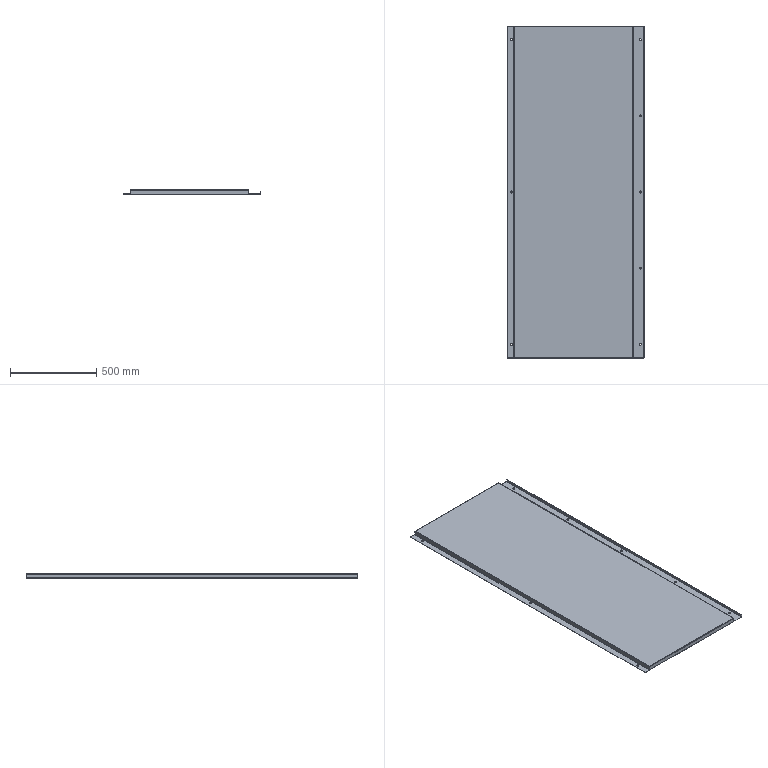Part | STEP file | Cover plate 2 | 1 solid | 78 faces | box 790 x 1920 x 25 mm | volume 2483939 mm3 | plane 40 | cylinder 30 | spline 8 | commonest cylinder face diameters 12 x16 2 x7 5 x7